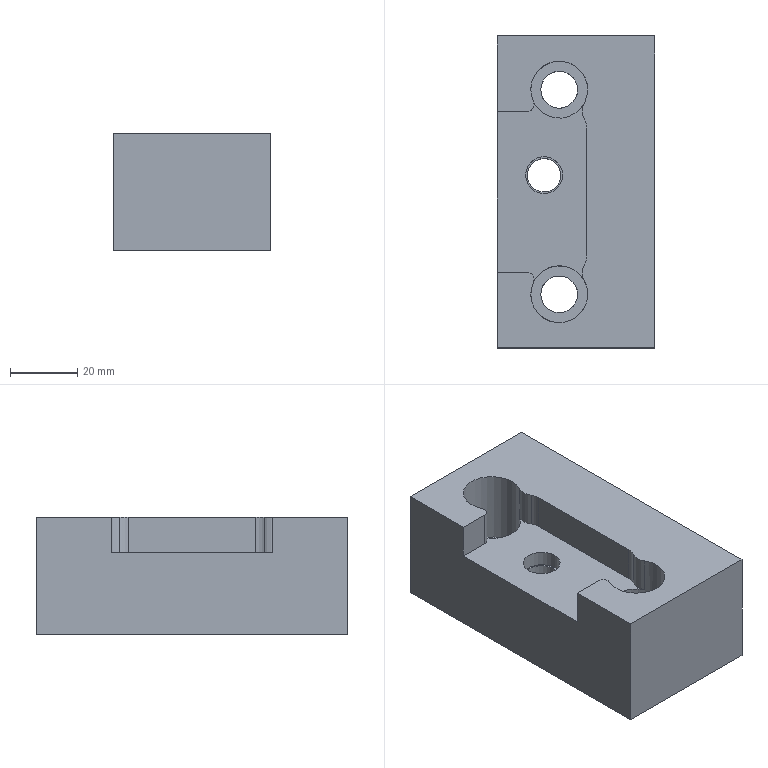Part | STEP file | lll_id4506_x_t | 1 solid | 25 faces | box 47 x 93 x 35 mm | volume 125345 mm3 | plane 13 | cylinder 12 | commonest cylinder face diameters 10 x5 11 x3 4 x2 17 x2
STEP:
#1=CARTESIAN_POINT('',(3748.75,-24.,0.));
#2=VERTEX_POINT('',#1);
#3=CARTESIAN_POINT('',(3748.75,-24.,-10.5));
#4=VERTEX_POINT('',#3);
#5=CARTESIAN_POINT('',(3748.75,-24.,-65.));
#6=DIRECTION('',(0.,0.,-1.));
#7=VECTOR('',#6,1.);
#8=LINE('',#5,#7);
#9=EDGE_CURVE('',#2,#4,#8,.T.);
#10=ORIENTED_EDGE('',*,*,#9,.T.);
#11=CARTESIAN_POINT('',(3748.75,24.,-10.5));
#12=VERTEX_POINT('',#11);
#13=CARTESIAN_POINT('',(3748.75,-0.9999,-10.5));
#14=DIRECTION('',(0.,-1.,0.));
#15=VECTOR('',#14,1.);
#16=LINE('',#13,#15);
#17=EDGE_CURVE('',#12,#4,#16,.T.);
#18=ORIENTED_EDGE('',*,*,#17,.F.);
#19=CARTESIAN_POINT('',(3748.75,24.,0.));
#20=VERTEX_POINT('',#19);
#21=CARTESIAN_POINT('',(3748.75,24.,-65.));
#22=DIRECTION('',(0.,0.,1.));
#23=VECTOR('',#22,1.);
#24=LINE('',#21,#23);
#25=EDGE_CURVE('',#12,#20,#24,.T.);
#26=ORIENTED_EDGE('',*,*,#25,.T.);
#27=CARTESIAN_POINT('',(3748.75,46.5,0.));
#28=VERTEX_POINT('',#27);
#29=CARTESIAN_POINT('',(3748.75,-7.,0.));
#30=DIRECTION('',(0.,-1.,0.));
#31=VECTOR('',#30,1.);
#32=LINE('',#29,#31);
#33=EDGE_CURVE('',#28,#20,#32,.T.);
#34=ORIENTED_EDGE('',*,*,#33,.F.);
#35=CARTESIAN_POINT('',(3748.75,46.5,-35.));
#36=VERTEX_POINT('',#35);
#37=CARTESIAN_POINT('',(3748.75,46.5,-65.));
#38=DIRECTION('',(0.,0.,-1.));
#39=VECTOR('',#38,1.);
#40=LINE('',#37,#39);
#41=EDGE_CURVE('',#28,#36,#40,.T.);
#42=ORIENTED_EDGE('',*,*,#41,.T.);
#43=CARTESIAN_POINT('',(3748.75,-46.5,-35.));
#44=VERTEX_POINT('',#43);
#45=CARTESIAN_POINT('',(3748.75,-7.,-35.));
#46=DIRECTION('',(0.,1.,0.));
#47=VECTOR('',#46,1.);
#48=LINE('',#45,#47);
#49=EDGE_CURVE('',#44,#36,#48,.T.);
#50=ORIENTED_EDGE('',*,*,#49,.F.);
#51=CARTESIAN_POINT('',(3748.75,-46.5,0.));
#52=VERTEX_POINT('',#51);
#53=CARTESIAN_POINT('',(3748.75,-46.5,-65.));
#54=DIRECTION('',(0.,0.,-1.));
#55=VECTOR('',#54,1.);
#56=LINE('',#53,#55);
#57=EDGE_CURVE('',#52,#44,#56,.T.);
#58=ORIENTED_EDGE('',*,*,#57,.F.);
#59=CARTESIAN_POINT('',(3748.75,-7.,0.));
#60=DIRECTION('',(0.,-1.,0.));
#61=VECTOR('',#60,1.);
#62=LINE('',#59,#61);
#63=EDGE_CURVE('',#2,#52,#62,.T.);
#64=ORIENTED_EDGE('',*,*,#63,.F.);
#65=EDGE_LOOP('',(#10,#18,#26,#34,#42,#50,#58,#64));
#66=FACE_OUTER_BOUND('',#65,.T.);
#67=CARTESIAN_POINT('',(3748.75,-7.,-65.));
#68=DIRECTION('',(-1.,0.,0.));
#69=DIRECTION('',(0.,0.,1.));
#70=AXIS2_PLACEMENT_3D('',#67,#68,#69);
#71=PLANE('',#70);
#72=ADVANCED_FACE('',(#66),#71,.T.);
#73=CARTESIAN_POINT('',(3768.25,5.,-15.));
#74=VERTEX_POINT('',#73);
#75=CARTESIAN_POINT('',(3762.75,5.,-15.));
#76=DIRECTION('',(0.,0.,-1.));
#77=DIRECTION('',(1.,0.,0.));
#78=AXIS2_PLACEMENT_3D('',#75,#76,#77);
#79=CIRCLE('',#78,5.5);
#80=EDGE_CURVE('',#74,#74,#79,.T.);
#81=ORIENTED_EDGE('',*,*,#80,.T.);
#82=EDGE_LOOP('',(#81));
#83=FACE_BOUND('',#82,.T.);
#84=CARTESIAN_POINT('',(3768.25,5.,-10.5));
#85=VERTEX_POINT('',#84);
#86=CARTESIAN_POINT('',(3762.75,5.,-10.5));
#87=DIRECTION('',(0.,0.,-1.));
#88=DIRECTION('',(1.,0.,0.));
#89=AXIS2_PLACEMENT_3D('',#86,#87,#88);
#90=CIRCLE('',#89,5.5);
#91=EDGE_CURVE('',#85,#85,#90,.T.);
#92=ORIENTED_EDGE('',*,*,#91,.F.);
#93=EDGE_LOOP('',(#92));
#94=FACE_BOUND('',#93,.T.);
#95=CARTESIAN_POINT('',(3762.75,5.,0.));
#96=DIRECTION('',(0.,0.,-1.));
#97=DIRECTION('',(1.,0.,0.));
#98=AXIS2_PLACEMENT_3D('',#95,#96,#97);
#99=CYLINDRICAL_SURFACE('',#98,5.5);
#100=ADVANCED_FACE('',(#83,#94),#99,.F.);
#101=CARTESIAN_POINT('',(3774.724,-26.451,0.));
#102=VERTEX_POINT('',#101);
#103=CARTESIAN_POINT('',(3759.57,-26.857,0.));
#104=VERTEX_POINT('',#103);
#105=CARTESIAN_POINT('',(3767.25,-30.5,0.));
#106=DIRECTION('',(0.,0.,-1.));
#107=DIRECTION('',(0.,-1.,0.));
#108=AXIS2_PLACEMENT_3D('',#105,#106,#107);
#109=CIRCLE('',#108,8.5);
#110=EDGE_CURVE('',#102,#104,#109,.T.);
#111=ORIENTED_EDGE('',*,*,#110,.T.);
#112=CARTESIAN_POINT('',(3757.763,-24.,0.));
#113=VERTEX_POINT('',#112);
#114=CARTESIAN_POINT('',(3757.763,-26.,0.));
#115=DIRECTION('',(0.,0.,1.));
#116=DIRECTION('',(1.,0.,0.));
#117=AXIS2_PLACEMENT_3D('',#114,#115,#116);
#118=CIRCLE('',#117,2.);
#119=EDGE_CURVE('',#104,#113,#118,.T.);
#120=ORIENTED_EDGE('',*,*,#119,.T.);
#121=CARTESIAN_POINT('',(3800.,-24.,0.));
#122=DIRECTION('',(-1.,0.,0.));
#123=VECTOR('',#122,1.);
#124=LINE('',#121,#123);
#125=EDGE_CURVE('',#113,#2,#124,.T.);
#126=ORIENTED_EDGE('',*,*,#125,.T.);
#127=ORIENTED_EDGE('',*,*,#63,.T.);
#128=CARTESIAN_POINT('',(3795.75,-46.5,0.));
#129=VERTEX_POINT('',#128);
#130=CARTESIAN_POINT('',(3800.,-46.5,0.));
#131=DIRECTION('',(1.,0.,0.));
#132=VECTOR('',#131,1.);
#133=LINE('',#130,#132);
#134=EDGE_CURVE('',#52,#129,#133,.T.);
#135=ORIENTED_EDGE('',*,*,#134,.T.);
#136=CARTESIAN_POINT('',(3795.75,46.5,0.));
#137=VERTEX_POINT('',#136);
#138=CARTESIAN_POINT('',(3795.75,-7.,0.));
#139=DIRECTION('',(0.,1.,0.));
#140=VECTOR('',#139,1.);
#141=LINE('',#138,#140);
#142=EDGE_CURVE('',#129,#137,#141,.T.);
#143=ORIENTED_EDGE('',*,*,#142,.T.);
#144=CARTESIAN_POINT('',(3800.,46.5,0.));
#145=DIRECTION('',(-1.,0.,0.));
#146=VECTOR('',#145,1.);
#147=LINE('',#144,#146);
#148=EDGE_CURVE('',#137,#28,#147,.T.);
#149=ORIENTED_EDGE('',*,*,#148,.T.);
#150=ORIENTED_EDGE('',*,*,#33,.T.);
#151=CARTESIAN_POINT('',(3757.763,24.,0.));
#152=VERTEX_POINT('',#151);
#153=CARTESIAN_POINT('',(3800.,24.,0.));
#154=DIRECTION('',(1.,0.,0.));
#155=VECTOR('',#154,1.);
#156=LINE('',#153,#155);
#157=EDGE_CURVE('',#20,#152,#156,.T.);
#158=ORIENTED_EDGE('',*,*,#157,.T.);
#159=CARTESIAN_POINT('',(3759.57,26.857,0.));
#160=VERTEX_POINT('',#159);
#161=CARTESIAN_POINT('',(3757.763,26.,0.));
#162=DIRECTION('',(0.,0.,1.));
#163=DIRECTION('',(1.,0.,0.));
#164=AXIS2_PLACEMENT_3D('',#161,#162,#163);
#165=CIRCLE('',#164,2.);
#166=EDGE_CURVE('',#152,#160,#165,.T.);
#167=ORIENTED_EDGE('',*,*,#166,.T.);
#168=CARTESIAN_POINT('',(3774.724,26.451,0.));
#169=VERTEX_POINT('',#168);
#170=CARTESIAN_POINT('',(3767.25,30.5,0.));
#171=DIRECTION('',(0.,0.,1.));
#172=DIRECTION('',(0.,1.,0.));
#173=AXIS2_PLACEMENT_3D('',#170,#171,#172);
#174=CIRCLE('',#173,8.5);
#175=EDGE_CURVE('',#169,#160,#174,.T.);
#176=ORIENTED_EDGE('',*,*,#175,.F.);
#177=CARTESIAN_POINT('',(3774.81,21.535,0.));
#178=VERTEX_POINT('',#177);
#179=CARTESIAN_POINT('',(3779.12,24.069,0.));
#180=DIRECTION('',(0.,0.,1.));
#181=DIRECTION('',(1.,0.,0.));
#182=AXIS2_PLACEMENT_3D('',#179,#180,#181);
#183=CIRCLE('',#182,5.);
#184=EDGE_CURVE('',#169,#178,#183,.T.);
#185=ORIENTED_EDGE('',*,*,#184,.T.);
#186=CARTESIAN_POINT('',(3775.5,19.,0.));
#187=VERTEX_POINT('',#186);
#188=CARTESIAN_POINT('',(3770.5,19.,0.));
#189=DIRECTION('',(0.,0.,-1.));
#190=DIRECTION('',(1.,0.,0.));
#191=AXIS2_PLACEMENT_3D('',#188,#189,#190);
#192=CIRCLE('',#191,5.);
#193=EDGE_CURVE('',#178,#187,#192,.T.);
#194=ORIENTED_EDGE('',*,*,#193,.T.);
#195=CARTESIAN_POINT('',(3775.5,-19.,0.));
#196=VERTEX_POINT('',#195);
#197=CARTESIAN_POINT('',(3775.5,-7.,0.));
#198=DIRECTION('',(0.,1.,0.));
#199=VECTOR('',#198,1.);
#200=LINE('',#197,#199);
#201=EDGE_CURVE('',#196,#187,#200,.T.);
#202=ORIENTED_EDGE('',*,*,#201,.F.);
#203=CARTESIAN_POINT('',(3774.81,-21.535,0.));
#204=VERTEX_POINT('',#203);
#205=CARTESIAN_POINT('',(3770.5,-19.,0.));
#206=DIRECTION('',(0.,0.,-1.));
#207=DIRECTION('',(1.,0.,0.));
#208=AXIS2_PLACEMENT_3D('',#205,#206,#207);
#209=CIRCLE('',#208,5.);
#210=EDGE_CURVE('',#196,#204,#209,.T.);
#211=ORIENTED_EDGE('',*,*,#210,.T.);
#212=CARTESIAN_POINT('',(3779.12,-24.069,0.));
#213=DIRECTION('',(0.,0.,1.));
#214=DIRECTION('',(1.,0.,0.));
#215=AXIS2_PLACEMENT_3D('',#212,#213,#214);
#216=CIRCLE('',#215,5.);
#217=EDGE_CURVE('',#204,#102,#216,.T.);
#218=ORIENTED_EDGE('',*,*,#217,.T.);
#219=EDGE_LOOP('',(#111,#120,#126,#127,#135,#143,#149,#150,#158,#167,#176,#185,#194,#202,#211,#218));
#220=FACE_OUTER_BOUND('',#219,.T.);
#221=CARTESIAN_POINT('',(3800.,-7.,0.));
#222=DIRECTION('',(0.,0.,1.));
#223=DIRECTION('',(1.,0.,0.));
#224=AXIS2_PLACEMENT_3D('',#221,#222,#223);
#225=PLANE('',#224);
#226=ADVANCED_FACE('',(#220),#225,.T.);
#227=CARTESIAN_POINT('',(3767.25,-25.,-35.));
#228=VERTEX_POINT('',#227);
#229=CARTESIAN_POINT('',(3767.25,-30.5,-35.));
#230=DIRECTION('',(0.,0.,-1.));
#231=DIRECTION('',(0.,1.,0.));
#232=AXIS2_PLACEMENT_3D('',#229,#230,#231);
#233=CIRCLE('',#232,5.5);
#234=EDGE_CURVE('',#228,#228,#233,.T.);
#235=ORIENTED_EDGE('',*,*,#234,.F.);
#236=EDGE_LOOP('',(#235));
#237=FACE_BOUND('',#236,.T.);
#238=CARTESIAN_POINT('',(3795.75,-46.5,-35.));
#239=VERTEX_POINT('',#238);
#240=CARTESIAN_POINT('',(3800.,-46.5,-35.));
#241=DIRECTION('',(-1.,0.,0.));
#242=VECTOR('',#241,1.);
#243=LINE('',#240,#242);
#244=EDGE_CURVE('',#239,#44,#243,.T.);
#245=ORIENTED_EDGE('',*,*,#244,.T.);
#246=ORIENTED_EDGE('',*,*,#49,.T.);
#247=CARTESIAN_POINT('',(3795.75,46.5,-35.));
#248=VERTEX_POINT('',#247);
#249=CARTESIAN_POINT('',(3800.,46.5,-35.));
#250=DIRECTION('',(1.,0.,0.));
#251=VECTOR('',#250,1.);
#252=LINE('',#249,#251);
#253=EDGE_CURVE('',#36,#248,#252,.T.);
#254=ORIENTED_EDGE('',*,*,#253,.T.);
#255=CARTESIAN_POINT('',(3795.75,-7.,-35.));
#256=DIRECTION('',(0.,-1.,0.));
#257=VECTOR('',#256,1.);
#258=LINE('',#255,#257);
#259=EDGE_CURVE('',#248,#239,#258,.T.);
#260=ORIENTED_EDGE('',*,*,#259,.T.);
#261=EDGE_LOOP('',(#245,#246,#254,#260));
#262=FACE_BOUND('',#261,.T.);
#263=CARTESIAN_POINT('',(3757.75,5.,-35.));
#264=VERTEX_POINT('',#263);
#265=CARTESIAN_POINT('',(3762.75,5.,-35.));
#266=DIRECTION('',(0.,0.,-1.));
#267=DIRECTION('',(-1.,0.,0.));
#268=AXIS2_PLACEMENT_3D('',#265,#266,#267);
#269=CIRCLE('',#268,5.);
#270=EDGE_CURVE('',#264,#264,#269,.T.);
#271=ORIENTED_EDGE('',*,*,#270,.F.);
#272=EDGE_LOOP('',(#271));
#273=FACE_BOUND('',#272,.T.);
#274=CARTESIAN_POINT('',(3767.25,25.,-35.));
#275=VERTEX_POINT('',#274);
#276=CARTESIAN_POINT('',(3767.25,30.5,-35.));
#277=DIRECTION('',(0.,0.,1.));
#278=DIRECTION('',(0.,-1.,0.));
#279=AXIS2_PLACEMENT_3D('',#276,#277,#278);
#280=CIRCLE('',#279,5.5);
#281=EDGE_CURVE('',#275,#275,#280,.T.);
#282=ORIENTED_EDGE('',*,*,#281,.T.);
#283=EDGE_LOOP('',(#282));
#284=FACE_BOUND('',#283,.T.);
#285=CARTESIAN_POINT('',(3800.,-7.,-35.));
#286=DIRECTION('',(0.,0.,-1.));
#287=DIRECTION('',(-1.,0.,0.));
#288=AXIS2_PLACEMENT_3D('',#285,#286,#287);
#289=PLANE('',#288);
#290=ADVANCED_FACE('',(#237,#262,#273,#284),#289,.T.);
#291=CARTESIAN_POINT('',(3761.75,-30.5,-22.));
#292=VERTEX_POINT('',#291);
#293=CARTESIAN_POINT('',(3767.25,-30.5,-22.));
#294=DIRECTION('',(0.,0.,1.));
#295=DIRECTION('',(-1.,0.,0.));
#296=AXIS2_PLACEMENT_3D('',#293,#294,#295);
#297=CIRCLE('',#296,5.5);
#298=EDGE_CURVE('',#292,#292,#297,.T.);
#299=ORIENTED_EDGE('',*,*,#298,.T.);
#300=EDGE_LOOP('',(#299));
#301=FACE_BOUND('',#300,.T.);
#302=ORIENTED_EDGE('',*,*,#234,.T.);
#303=EDGE_LOOP('',(#302));
#304=FACE_BOUND('',#303,.T.);
#305=CARTESIAN_POINT('',(3767.25,-30.5,-20.));
#306=DIRECTION('',(0.,0.,-1.));
#307=DIRECTION('',(-1.,0.,0.));
#308=AXIS2_PLACEMENT_3D('',#305,#306,#307);
#309=CYLINDRICAL_SURFACE('',#308,5.5);
#310=ADVANCED_FACE('',(#301,#304),#309,.F.);
#311=CARTESIAN_POINT('',(3767.75,5.,-15.));
#312=VERTEX_POINT('',#311);
#313=CARTESIAN_POINT('',(3762.75,5.,-15.));
#314=DIRECTION('',(0.,0.,-1.));
#315=DIRECTION('',(1.,0.,0.));
#316=AXIS2_PLACEMENT_3D('',#313,#314,#315);
#317=CIRCLE('',#316,5.);
#318=EDGE_CURVE('',#312,#312,#317,.T.);
#319=ORIENTED_EDGE('',*,*,#318,.F.);
#320=EDGE_LOOP('',(#319));
#321=FACE_BOUND('',#320,.T.);
#322=ORIENTED_EDGE('',*,*,#270,.T.);
#323=EDGE_LOOP('',(#322));
#324=FACE_BOUND('',#323,.T.);
#325=CARTESIAN_POINT('',(3762.75,5.,-20.));
#326=DIRECTION('',(0.,0.,-1.));
#327=DIRECTION('',(1.,0.,0.));
#328=AXIS2_PLACEMENT_3D('',#325,#326,#327);
#329=CYLINDRICAL_SURFACE('',#328,5.);
#330=ADVANCED_FACE('',(#321,#324),#329,.F.);
#331=ORIENTED_EDGE('',*,*,#80,.F.);
#332=EDGE_LOOP('',(#331));
#333=FACE_BOUND('',#332,.T.);
#334=ORIENTED_EDGE('',*,*,#318,.T.);
#335=EDGE_LOOP('',(#334));
#336=FACE_BOUND('',#335,.T.);
#337=CARTESIAN_POINT('',(3762.75,5.,-15.));
#338=DIRECTION('',(0.,0.,-1.));
#339=DIRECTION('',(1.,0.,0.));
#340=AXIS2_PLACEMENT_3D('',#337,#338,#339);
#341=PLANE('',#340);
#342=ADVANCED_FACE('',(#333,#336),#341,.F.);
#343=ORIENTED_EDGE('',*,*,#259,.F.);
#344=CARTESIAN_POINT('',(3795.75,46.5,-65.));
#345=DIRECTION('',(0.,0.,-1.));
#346=VECTOR('',#345,1.);
#347=LINE('',#344,#346);
#348=EDGE_CURVE('',#137,#248,#347,.T.);
#349=ORIENTED_EDGE('',*,*,#348,.F.);
#350=ORIENTED_EDGE('',*,*,#142,.F.);
#351=CARTESIAN_POINT('',(3795.75,-46.5,-65.));
#352=DIRECTION('',(0.,0.,-1.));
#353=VECTOR('',#352,1.);
#354=LINE('',#351,#353);
#355=EDGE_CURVE('',#129,#239,#354,.T.);
#356=ORIENTED_EDGE('',*,*,#355,.T.);
#357=EDGE_LOOP('',(#343,#349,#350,#356));
#358=FACE_OUTER_BOUND('',#357,.T.);
#359=CARTESIAN_POINT('',(3795.75,-7.,-65.));
#360=DIRECTION('',(1.,0.,0.));
#361=DIRECTION('',(0.,0.,-1.));
#362=AXIS2_PLACEMENT_3D('',#359,#360,#361);
#363=PLANE('',#362);
#364=ADVANCED_FACE('',(#358),#363,.T.);
#365=ORIENTED_EDGE('',*,*,#253,.F.);
#366=ORIENTED_EDGE('',*,*,#41,.F.);
#367=ORIENTED_EDGE('',*,*,#148,.F.);
#368=ORIENTED_EDGE('',*,*,#348,.T.);
#369=EDGE_LOOP('',(#365,#366,#367,#368));
#370=FACE_OUTER_BOUND('',#369,.T.);
#371=CARTESIAN_POINT('',(3800.,46.5,-65.));
#372=DIRECTION('',(0.,1.,0.));
#373=DIRECTION('',(0.,0.,-1.));
#374=AXIS2_PLACEMENT_3D('',#371,#372,#373);
#375=PLANE('',#374);
#376=ADVANCED_FACE('',(#370),#375,.T.);
#377=ORIENTED_EDGE('',*,*,#134,.F.);
#378=ORIENTED_EDGE('',*,*,#57,.T.);
#379=ORIENTED_EDGE('',*,*,#244,.F.);
#380=ORIENTED_EDGE('',*,*,#355,.F.);
#381=EDGE_LOOP('',(#377,#378,#379,#380));
#382=FACE_OUTER_BOUND('',#381,.T.);
#383=CARTESIAN_POINT('',(3800.,-46.5,-65.));
#384=DIRECTION('',(0.,-1.,0.));
#385=DIRECTION('',(0.,0.,1.));
#386=AXIS2_PLACEMENT_3D('',#383,#384,#385);
#387=PLANE('',#386);
#388=ADVANCED_FACE('',(#382),#387,.T.);
#389=ORIENTED_EDGE('',*,*,#298,.F.);
#390=EDGE_LOOP('',(#389));
#391=FACE_BOUND('',#390,.T.);
#392=CARTESIAN_POINT('',(3775.75,-30.5,-22.));
#393=VERTEX_POINT('',#392);
#394=CARTESIAN_POINT('',(3767.25,-30.5,-22.));
#395=DIRECTION('',(0.,0.,-1.));
#396=DIRECTION('',(1.,0.,0.));
#397=AXIS2_PLACEMENT_3D('',#394,#395,#396);
#398=CIRCLE('',#397,8.5);
#399=EDGE_CURVE('',#393,#393,#398,.T.);
#400=ORIENTED_EDGE('',*,*,#399,.F.);
#401=EDGE_LOOP('',(#400));
#402=FACE_BOUND('',#401,.T.);
#403=CARTESIAN_POINT('',(3772.25,-30.5,-22.));
#404=DIRECTION('',(0.,0.,-1.));
#405=DIRECTION('',(-1.,0.,0.));
#406=AXIS2_PLACEMENT_3D('',#403,#404,#405);
#407=PLANE('',#406);
#408=ADVANCED_FACE('',(#391,#402),#407,.F.);
#409=ORIENTED_EDGE('',*,*,#399,.T.);
#410=EDGE_LOOP('',(#409));
#411=FACE_BOUND('',#410,.T.);
#412=CARTESIAN_POINT('',(3759.57,-26.857,-10.5));
#413=VERTEX_POINT('',#412);
#414=CARTESIAN_POINT('',(3774.724,-26.451,-10.5));
#415=VERTEX_POINT('',#414);
#416=CARTESIAN_POINT('',(3767.25,-30.5,-10.5));
#417=DIRECTION('',(0.,0.,-1.));
#418=DIRECTION('',(1.,0.,0.));
#419=AXIS2_PLACEMENT_3D('',#416,#417,#418);
#420=CIRCLE('',#419,8.5);
#421=EDGE_CURVE('',#413,#415,#420,.T.);
#422=ORIENTED_EDGE('',*,*,#421,.F.);
#423=CARTESIAN_POINT('',(3759.57,-26.857,-20.));
#424=DIRECTION('',(0.,0.,1.));
#425=VECTOR('',#424,1.);
#426=LINE('',#423,#425);
#427=EDGE_CURVE('',#413,#104,#426,.T.);
#428=ORIENTED_EDGE('',*,*,#427,.T.);
#429=ORIENTED_EDGE('',*,*,#110,.F.);
#430=CARTESIAN_POINT('',(3774.724,-26.451,-20.));
#431=DIRECTION('',(0.,0.,-1.));
#432=VECTOR('',#431,1.);
#433=LINE('',#430,#432);
#434=EDGE_CURVE('',#102,#415,#433,.T.);
#435=ORIENTED_EDGE('',*,*,#434,.T.);
#436=EDGE_LOOP('',(#422,#428,#429,#435));
#437=FACE_BOUND('',#436,.T.);
#438=CARTESIAN_POINT('',(3767.25,-30.5,-20.));
#439=DIRECTION('',(0.,0.,1.));
#440=DIRECTION('',(1.,0.,0.));
#441=AXIS2_PLACEMENT_3D('',#438,#439,#440);
#442=CYLINDRICAL_SURFACE('',#441,8.5);
#443=ADVANCED_FACE('',(#411,#437),#442,.F.);
#444=CARTESIAN_POINT('',(3758.75,30.5,-22.));
#445=VERTEX_POINT('',#444);
#446=CARTESIAN_POINT('',(3767.25,30.5,-22.));
#447=DIRECTION('',(0.,0.,1.));
#448=DIRECTION('',(-1.,0.,0.));
#449=AXIS2_PLACEMENT_3D('',#446,#447,#448);
#450=CIRCLE('',#449,8.5);
#451=EDGE_CURVE('',#445,#445,#450,.T.);
#452=ORIENTED_EDGE('',*,*,#451,.F.);
#453=EDGE_LOOP('',(#452));
#454=FACE_BOUND('',#453,.T.);
#455=ORIENTED_EDGE('',*,*,#175,.T.);
#456=CARTESIAN_POINT('',(3759.57,26.857,-10.5));
#457=VERTEX_POINT('',#456);
#458=CARTESIAN_POINT('',(3759.57,26.857,-20.));
#459=DIRECTION('',(0.,0.,-1.));
#460=VECTOR('',#459,1.);
#461=LINE('',#458,#460);
#462=EDGE_CURVE('',#160,#457,#461,.T.);
#463=ORIENTED_EDGE('',*,*,#462,.T.);
#464=CARTESIAN_POINT('',(3774.724,26.451,-10.5));
#465=VERTEX_POINT('',#464);
#466=CARTESIAN_POINT('',(3767.25,30.5,-10.5));
#467=DIRECTION('',(0.,0.,1.));
#468=DIRECTION('',(1.,0.,0.));
#469=AXIS2_PLACEMENT_3D('',#466,#467,#468);
#470=CIRCLE('',#469,8.5);
#471=EDGE_CURVE('',#457,#465,#470,.T.);
#472=ORIENTED_EDGE('',*,*,#471,.T.);
#473=CARTESIAN_POINT('',(3774.724,26.451,-20.));
#474=DIRECTION('',(0.,0.,1.));
#475=VECTOR('',#474,1.);
#476=LINE('',#473,#475);
#477=EDGE_CURVE('',#465,#169,#476,.T.);
#478=ORIENTED_EDGE('',*,*,#477,.T.);
#479=EDGE_LOOP('',(#455,#463,#472,#478));
#480=FACE_BOUND('',#479,.T.);
#481=CARTESIAN_POINT('',(3767.25,30.5,-20.));
#482=DIRECTION('',(0.,0.,1.));
#483=DIRECTION('',(1.,0.,0.));
#484=AXIS2_PLACEMENT_3D('',#481,#482,#483);
#485=CYLINDRICAL_SURFACE('',#484,8.5);
#486=ADVANCED_FACE('',(#454,#480),#485,.F.);
#487=CARTESIAN_POINT('',(3761.75,30.5,-22.));
#488=VERTEX_POINT('',#487);
#489=CARTESIAN_POINT('',(3767.25,30.5,-22.));
#490=DIRECTION('',(0.,0.,-1.));
#491=DIRECTION('',(-1.,0.,0.));
#492=AXIS2_PLACEMENT_3D('',#489,#490,#491);
#493=CIRCLE('',#492,5.5);
#494=EDGE_CURVE('',#488,#488,#493,.T.);
#495=ORIENTED_EDGE('',*,*,#494,.F.);
#496=EDGE_LOOP('',(#495));
#497=FACE_BOUND('',#496,.T.);
#498=ORIENTED_EDGE('',*,*,#281,.F.);
#499=EDGE_LOOP('',(#498));
#500=FACE_BOUND('',#499,.T.);
#501=CARTESIAN_POINT('',(3767.25,30.5,-20.));
#502=DIRECTION('',(0.,0.,-1.));
#503=DIRECTION('',(-1.,0.,0.));
#504=AXIS2_PLACEMENT_3D('',#501,#502,#503);
#505=CYLINDRICAL_SURFACE('',#504,5.5);
#506=ADVANCED_FACE('',(#497,#500),#505,.F.);
#507=ORIENTED_EDGE('',*,*,#494,.T.);
#508=EDGE_LOOP('',(#507));
#509=FACE_BOUND('',#508,.T.);
#510=ORIENTED_EDGE('',*,*,#451,.T.);
#511=EDGE_LOOP('',(#510));
#512=FACE_BOUND('',#511,.T.);
#513=CARTESIAN_POINT('',(3772.25,30.5,-22.));
#514=DIRECTION('',(0.,0.,-1.));
#515=DIRECTION('',(-1.,0.,0.));
#516=AXIS2_PLACEMENT_3D('',#513,#514,#515);
#517=PLANE('',#516);
#518=ADVANCED_FACE('',(#509,#512),#517,.F.);
#519=ORIENTED_EDGE('',*,*,#125,.F.);
#520=CARTESIAN_POINT('',(3757.763,-24.,-10.5));
#521=VERTEX_POINT('',#520);
#522=CARTESIAN_POINT('',(3757.763,-24.,12.5));
#523=DIRECTION('',(0.,0.,-1.));
#524=VECTOR('',#523,1.);
#525=LINE('',#522,#524);
#526=EDGE_CURVE('',#113,#521,#525,.T.);
#527=ORIENTED_EDGE('',*,*,#526,.T.);
#528=CARTESIAN_POINT('',(3794.,-24.,-10.5));
#529=DIRECTION('',(1.,0.,0.));
#530=VECTOR('',#529,1.);
#531=LINE('',#528,#530);
#532=EDGE_CURVE('',#4,#521,#531,.T.);
#533=ORIENTED_EDGE('',*,*,#532,.F.);
#534=ORIENTED_EDGE('',*,*,#9,.F.);
#535=EDGE_LOOP('',(#519,#527,#533,#534));
#536=FACE_OUTER_BOUND('',#535,.T.);
#537=CARTESIAN_POINT('',(3794.,-24.,12.5));
#538=DIRECTION('',(0.,1.,0.));
#539=DIRECTION('',(0.,0.,1.));
#540=AXIS2_PLACEMENT_3D('',#537,#538,#539);
#541=PLANE('',#540);
#542=ADVANCED_FACE('',(#536),#541,.T.);
#543=CARTESIAN_POINT('',(3775.5,19.,-10.5));
#544=VERTEX_POINT('',#543);
#545=CARTESIAN_POINT('',(3775.5,-19.,-10.5));
#546=VERTEX_POINT('',#545);
#547=CARTESIAN_POINT('',(3775.5,0.00007422,-10.5));
#548=DIRECTION('',(0.,-1.,0.));
#549=VECTOR('',#548,1.);
#550=LINE('',#547,#549);
#551=EDGE_CURVE('',#544,#546,#550,.T.);
#552=ORIENTED_EDGE('',*,*,#551,.T.);
#553=CARTESIAN_POINT('',(3775.5,-19.,12.5));
#554=DIRECTION('',(0.,0.,1.));
#555=VECTOR('',#554,1.);
#556=LINE('',#553,#555);
#557=EDGE_CURVE('',#546,#196,#556,.T.);
#558=ORIENTED_EDGE('',*,*,#557,.T.);
#559=ORIENTED_EDGE('',*,*,#201,.T.);
#560=CARTESIAN_POINT('',(3775.5,19.,12.5));
#561=DIRECTION('',(0.,0.,-1.));
#562=VECTOR('',#561,1.);
#563=LINE('',#560,#562);
#564=EDGE_CURVE('',#187,#544,#563,.T.);
#565=ORIENTED_EDGE('',*,*,#564,.T.);
#566=EDGE_LOOP('',(#552,#558,#559,#565));
#567=FACE_OUTER_BOUND('',#566,.T.);
#568=CARTESIAN_POINT('',(3775.5,0.00007422,12.5));
#569=DIRECTION('',(1.,0.,0.));
#570=DIRECTION('',(0.,0.,-1.));
#571=AXIS2_PLACEMENT_3D('',#568,#569,#570);
#572=PLANE('',#571);
#573=ADVANCED_FACE('',(#567),#572,.F.);
#574=ORIENTED_EDGE('',*,*,#421,.T.);
#575=CARTESIAN_POINT('',(3774.81,-21.535,-10.5));
#576=VERTEX_POINT('',#575);
#577=CARTESIAN_POINT('',(3779.12,-24.069,-10.5));
#578=DIRECTION('',(0.,0.,-1.));
#579=DIRECTION('',(1.,0.,0.));
#580=AXIS2_PLACEMENT_3D('',#577,#578,#579);
#581=CIRCLE('',#580,5.);
#582=EDGE_CURVE('',#415,#576,#581,.T.);
#583=ORIENTED_EDGE('',*,*,#582,.T.);
#584=CARTESIAN_POINT('',(3770.5,-19.,-10.5));
#585=DIRECTION('',(0.,0.,1.));
#586=DIRECTION('',(1.,0.,0.));
#587=AXIS2_PLACEMENT_3D('',#584,#585,#586);
#588=CIRCLE('',#587,5.);
#589=EDGE_CURVE('',#576,#546,#588,.T.);
#590=ORIENTED_EDGE('',*,*,#589,.T.);
#591=ORIENTED_EDGE('',*,*,#551,.F.);
#592=CARTESIAN_POINT('',(3774.81,21.535,-10.5));
#593=VERTEX_POINT('',#592);
#594=CARTESIAN_POINT('',(3770.5,19.,-10.5));
#595=DIRECTION('',(0.,0.,1.));
#596=DIRECTION('',(1.,0.,0.));
#597=AXIS2_PLACEMENT_3D('',#594,#595,#596);
#598=CIRCLE('',#597,5.);
#599=EDGE_CURVE('',#544,#593,#598,.T.);
#600=ORIENTED_EDGE('',*,*,#599,.T.);
#601=CARTESIAN_POINT('',(3779.12,24.069,-10.5));
#602=DIRECTION('',(0.,0.,-1.));
#603=DIRECTION('',(1.,0.,0.));
#604=AXIS2_PLACEMENT_3D('',#601,#602,#603);
#605=CIRCLE('',#604,5.);
#606=EDGE_CURVE('',#593,#465,#605,.T.);
#607=ORIENTED_EDGE('',*,*,#606,.T.);
#608=ORIENTED_EDGE('',*,*,#471,.F.);
#609=CARTESIAN_POINT('',(3757.763,24.,-10.5));
#610=VERTEX_POINT('',#609);
#611=CARTESIAN_POINT('',(3757.763,26.,-10.5));
#612=DIRECTION('',(0.,0.,-1.));
#613=DIRECTION('',(1.,0.,0.));
#614=AXIS2_PLACEMENT_3D('',#611,#612,#613);
#615=CIRCLE('',#614,2.);
#616=EDGE_CURVE('',#457,#610,#615,.T.);
#617=ORIENTED_EDGE('',*,*,#616,.T.);
#618=CARTESIAN_POINT('',(3794.,24.,-10.5));
#619=DIRECTION('',(-1.,0.,0.));
#620=VECTOR('',#619,1.);
#621=LINE('',#618,#620);
#622=EDGE_CURVE('',#610,#12,#621,.T.);
#623=ORIENTED_EDGE('',*,*,#622,.T.);
#624=ORIENTED_EDGE('',*,*,#17,.T.);
#625=ORIENTED_EDGE('',*,*,#532,.T.);
#626=CARTESIAN_POINT('',(3757.763,-26.,-10.5));
#627=DIRECTION('',(0.,0.,-1.));
#628=DIRECTION('',(1.,0.,0.));
#629=AXIS2_PLACEMENT_3D('',#626,#627,#628);
#630=CIRCLE('',#629,2.);
#631=EDGE_CURVE('',#521,#413,#630,.T.);
#632=ORIENTED_EDGE('',*,*,#631,.T.);
#633=EDGE_LOOP('',(#574,#583,#590,#591,#600,#607,#608,#617,#623,#624,#625,#632));
#634=FACE_BOUND('',#633,.T.);
#635=ORIENTED_EDGE('',*,*,#91,.T.);
#636=EDGE_LOOP('',(#635));
#637=FACE_BOUND('',#636,.T.);
#638=CARTESIAN_POINT('',(7344.751,-0.9999,-10.5));
#639=DIRECTION('',(0.,0.,1.));
#640=DIRECTION('',(1.,0.,0.));
#641=AXIS2_PLACEMENT_3D('',#638,#639,#640);
#642=PLANE('',#641);
#643=ADVANCED_FACE('',(#634,#637),#642,.T.);
#644=ORIENTED_EDGE('',*,*,#622,.F.);
#645=CARTESIAN_POINT('',(3757.763,24.,12.5));
#646=DIRECTION('',(0.,0.,1.));
#647=VECTOR('',#646,1.);
#648=LINE('',#645,#647);
#649=EDGE_CURVE('',#610,#152,#648,.T.);
#650=ORIENTED_EDGE('',*,*,#649,.T.);
#651=ORIENTED_EDGE('',*,*,#157,.F.);
#652=ORIENTED_EDGE('',*,*,#25,.F.);
#653=EDGE_LOOP('',(#644,#650,#651,#652));
#654=FACE_OUTER_BOUND('',#653,.T.);
#655=CARTESIAN_POINT('',(3794.,24.,12.5));
#656=DIRECTION('',(0.,-1.,0.));
#657=DIRECTION('',(0.,0.,1.));
#658=AXIS2_PLACEMENT_3D('',#655,#656,#657);
#659=PLANE('',#658);
#660=ADVANCED_FACE('',(#654),#659,.T.);
#661=ORIENTED_EDGE('',*,*,#589,.F.);
#662=CARTESIAN_POINT('',(3774.81,-21.535,12.5));
#663=DIRECTION('',(0.,0.,1.));
#664=VECTOR('',#663,1.);
#665=LINE('',#662,#664);
#666=EDGE_CURVE('',#576,#204,#665,.T.);
#667=ORIENTED_EDGE('',*,*,#666,.T.);
#668=ORIENTED_EDGE('',*,*,#210,.F.);
#669=ORIENTED_EDGE('',*,*,#557,.F.);
#670=EDGE_LOOP('',(#661,#667,#668,#669));
#671=FACE_OUTER_BOUND('',#670,.T.);
#672=CARTESIAN_POINT('',(3770.5,-19.,12.5));
#673=DIRECTION('',(0.,0.,-1.));
#674=DIRECTION('',(-1.,0.,0.));
#675=AXIS2_PLACEMENT_3D('',#672,#673,#674);
#676=CYLINDRICAL_SURFACE('',#675,5.);
#677=ADVANCED_FACE('',(#671),#676,.F.);
#678=ORIENTED_EDGE('',*,*,#193,.F.);
#679=CARTESIAN_POINT('',(3774.81,21.535,12.5));
#680=DIRECTION('',(0.,0.,-1.));
#681=VECTOR('',#680,1.);
#682=LINE('',#679,#681);
#683=EDGE_CURVE('',#178,#593,#682,.T.);
#684=ORIENTED_EDGE('',*,*,#683,.T.);
#685=ORIENTED_EDGE('',*,*,#599,.F.);
#686=ORIENTED_EDGE('',*,*,#564,.F.);
#687=EDGE_LOOP('',(#678,#684,#685,#686));
#688=FACE_OUTER_BOUND('',#687,.T.);
#689=CARTESIAN_POINT('',(3770.5,19.,12.5));
#690=DIRECTION('',(0.,0.,1.));
#691=DIRECTION('',(1.,0.,0.));
#692=AXIS2_PLACEMENT_3D('',#689,#690,#691);
#693=CYLINDRICAL_SURFACE('',#692,5.);
#694=ADVANCED_FACE('',(#688),#693,.F.);
#695=ORIENTED_EDGE('',*,*,#606,.F.);
#696=ORIENTED_EDGE('',*,*,#683,.F.);
#697=ORIENTED_EDGE('',*,*,#184,.F.);
#698=ORIENTED_EDGE('',*,*,#477,.F.);
#699=EDGE_LOOP('',(#695,#696,#697,#698));
#700=FACE_OUTER_BOUND('',#699,.T.);
#701=CARTESIAN_POINT('',(3779.12,24.069,12.5));
#702=DIRECTION('',(0.,0.,1.));
#703=DIRECTION('',(1.,0.,0.));
#704=AXIS2_PLACEMENT_3D('',#701,#702,#703);
#705=CYLINDRICAL_SURFACE('',#704,5.);
#706=ADVANCED_FACE('',(#700),#705,.T.);
#707=ORIENTED_EDGE('',*,*,#582,.F.);
#708=ORIENTED_EDGE('',*,*,#434,.F.);
#709=ORIENTED_EDGE('',*,*,#217,.F.);
#710=ORIENTED_EDGE('',*,*,#666,.F.);
#711=EDGE_LOOP('',(#707,#708,#709,#710));
#712=FACE_OUTER_BOUND('',#711,.T.);
#713=CARTESIAN_POINT('',(3779.12,-24.069,-20.));
#714=DIRECTION('',(0.,0.,1.));
#715=DIRECTION('',(1.,0.,0.));
#716=AXIS2_PLACEMENT_3D('',#713,#714,#715);
#717=CYLINDRICAL_SURFACE('',#716,5.);
#718=ADVANCED_FACE('',(#712),#717,.T.);
#719=ORIENTED_EDGE('',*,*,#119,.F.);
#720=ORIENTED_EDGE('',*,*,#427,.F.);
#721=ORIENTED_EDGE('',*,*,#631,.F.);
#722=ORIENTED_EDGE('',*,*,#526,.F.);
#723=EDGE_LOOP('',(#719,#720,#721,#722));
#724=FACE_OUTER_BOUND('',#723,.T.);
#725=CARTESIAN_POINT('',(3757.763,-26.,-20.));
#726=DIRECTION('',(0.,0.,1.));
#727=DIRECTION('',(1.,0.,0.));
#728=AXIS2_PLACEMENT_3D('',#725,#726,#727);
#729=CYLINDRICAL_SURFACE('',#728,2.);
#730=ADVANCED_FACE('',(#724),#729,.T.);
#731=ORIENTED_EDGE('',*,*,#166,.F.);
#732=ORIENTED_EDGE('',*,*,#649,.F.);
#733=ORIENTED_EDGE('',*,*,#616,.F.);
#734=ORIENTED_EDGE('',*,*,#462,.F.);
#735=EDGE_LOOP('',(#731,#732,#733,#734));
#736=FACE_OUTER_BOUND('',#735,.T.);
#737=CARTESIAN_POINT('',(3757.763,26.,-20.));
#738=DIRECTION('',(0.,0.,1.));
#739=DIRECTION('',(1.,0.,0.));
#740=AXIS2_PLACEMENT_3D('',#737,#738,#739);
#741=CYLINDRICAL_SURFACE('',#740,2.);
#742=ADVANCED_FACE('',(#736),#741,.T.);
#743=CLOSED_SHELL('',(#72,#100,#226,#290,#310,#330,#342,#364,#376,#388,#408,#443,#486,#506,#518,#542,#573,#643,#660,#677,#694,#706,#718,#730,#742));
#744=MANIFOLD_SOLID_BREP('',#743);
#745=(LENGTH_UNIT()NAMED_UNIT(*)SI_UNIT(.MILLI.,.METRE.));
#746=UNCERTAINTY_MEASURE_WITH_UNIT(LENGTH_MEASURE(0.00002),#745,'','');
#747=(NAMED_UNIT(*)PLANE_ANGLE_UNIT()SI_UNIT($,.RADIAN.));
#748=PLANE_ANGLE_MEASURE_WITH_UNIT(PLANE_ANGLE_MEASURE(0.01745),#747);
#749=DIMENSIONAL_EXPONENTS(0.,0.,0.,0.,0.,0.,0.);
#750=(CONVERSION_BASED_UNIT('DEGREE',#748)NAMED_UNIT(#749)PLANE_ANGLE_UNIT());
#751=(NAMED_UNIT(*)SI_UNIT($,.STERADIAN.)SOLID_ANGLE_UNIT());
#752=(GEOMETRIC_REPRESENTATION_CONTEXT(3)GLOBAL_UNCERTAINTY_ASSIGNED_CONTEXT((#746))GLOBAL_UNIT_ASSIGNED_CONTEXT((#745,#750,#751))REPRESENTATION_CONTEXT('',''));
#753=ADVANCED_BREP_SHAPE_REPRESENTATION('',(#744),#752);